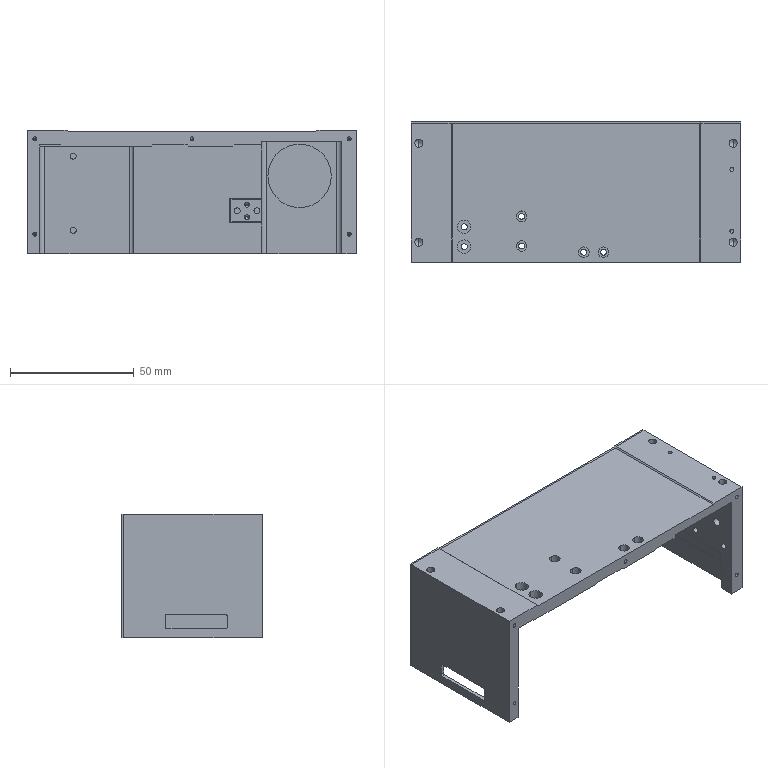NC program | NX | posted with a generic post | part box 133 x 56.74 x 50 mm
Lines 1 to 301 of 22463:
N10 G17 G21 G94 G90
(FLOOR_WALL_COPY_1 , TOOL : D10)
N12 T10 M6
N14 G54
N16 G17 G0 G90 X-74.5 Y28.367 B0. C0. S9500 M3
N18 G43 Z30. H10
N20 Z7.51
N22 G94 G1 Z4.51 F1250.
N24 X-71.5
N26 X71.5
N28 Y20.833
N30 X-71.5
N32 Y13.299
N34 X71.5
N36 Y5.765
N38 X-71.5
N40 Y-1.768
N42 X71.5
N44 Y-9.302
N46 X-71.5
N48 Y-16.836
N50 X71.5
N52 Y-24.37
N54 X-71.5
N56 X-74.5
N58 Z7.51
N60 G0 Z30.
N62 Y28.367
N64 Z7.02
N66 G1 Z4.02
N68 X-71.5
N70 X71.5
N72 Y20.833
N74 X-71.5
N76 Y13.299
N78 X71.5
N80 Y5.765
N82 X-71.5
N84 Y-1.768
N86 X71.5
N88 Y-9.302
N90 X-71.5
N92 Y-16.836
N94 X71.5
N96 Y-24.37
N98 X-71.5
N100 X-74.5
N102 Z7.02
N104 G0 Z30.
N106 Y28.367
N108 Z6.53
N110 G1 Z3.53
N112 X-71.5
N114 X71.5
N116 Y20.833
N118 X-71.5
N120 Y13.299
N122 X71.5
N124 Y5.765
N126 X-71.5
N128 Y-1.768
N130 X71.5
N132 Y-9.302
N134 X-71.5
N136 Y-16.836
N138 X71.5
N140 Y-24.37
N142 X-71.5
N144 X-74.5
N146 Z6.53
N148 G0 Z30.
N150 Y28.367
N152 Z6.04
N154 G1 Z3.04
N156 X-71.5
N158 X71.5
N160 Y20.833
N162 X-71.5
N164 Y13.299
N166 X71.5
N168 Y5.765
N170 X-71.5
N172 Y-1.768
N174 X71.5
N176 Y-9.302
N178 X-71.5
N180 Y-16.836
N182 X71.5
N184 Y-24.37
N186 X-71.5
N188 X-74.5
N190 Z6.04
N192 G0 Z30.
N194 Y28.367
N196 Z5.55
N198 G1 Z2.55
N200 X-71.5
N202 X71.5
N204 Y20.833
N206 X-71.5
N208 Y13.299
N210 X71.5
N212 Y5.765
N214 X-71.5
N216 Y-1.768
N218 X71.5
N220 Y-9.302
N222 X-71.5
N224 Y-16.836
N226 X71.5
N228 Y-24.37
N230 X-71.5
N232 X-74.5
N234 Z5.55
N236 G0 Z30.
N238 Y28.367
N240 Z5.06
N242 G1 Z2.06
N244 X-71.5
N246 X71.5
N248 Y20.833
N250 X-71.5
N252 Y13.299
N254 X71.5
N256 Y5.765
N258 X-71.5
N260 Y-1.768
N262 X71.5
N264 Y-9.302
N266 X-71.5
N268 Y-16.836
N270 X71.5
N272 Y-24.37
N274 X-71.5
N276 X-74.5
N278 Z5.06
N280 G0 Z30.
N282 Y28.367
N284 Z4.57
N286 G1 Z1.57
N288 X-71.5
N290 X71.5
N292 Y20.833
N294 X-71.5
N296 Y13.299
N298 X71.5
N300 Y5.765
N302 X-71.5
N304 Y-1.768
N306 X71.5
N308 Y-9.302
N310 X-71.5
N312 Y-16.836
N314 X71.5
N316 Y-24.37
N318 X-71.5
N320 X-74.5
N322 Z4.57
N324 G0 Z30.
N326 Y28.367
N328 Z4.08
N330 G1 Z1.08
N332 X-71.5
N334 X71.5
N336 Y20.833
N338 X-71.5
N340 Y13.299
N342 X71.5
N344 Y5.765
N346 X-71.5
N348 Y-1.768
N350 X71.5
N352 Y-9.302
N354 X-71.5
N356 Y-16.836
N358 X71.5
N360 Y-24.37
N362 X-71.5
N364 X-74.5
N366 Z4.08
N368 G0 Z30.
N370 Y28.367
N372 Z3.59
N374 G1 Z0.59
N376 X-71.5
N378 X71.5
N380 Y20.833
N382 X-71.5
N384 Y13.299
N386 X71.5
N388 Y5.765
N390 X-71.5
N392 Y-1.768
N394 X71.5
N396 Y-9.302
N398 X-71.5
N400 Y-16.836
N402 X71.5
N404 Y-24.37
N406 X-71.5
N408 X-74.5
N410 Z3.59
N412 G0 Z30.
N414 Y28.367
N416 Z3.1
N418 G1 Z0.1
N420 X-71.5
N422 X71.5
N424 Y20.833
N426 X-71.5
N428 Y13.299
N430 X71.5
N432 Y5.765
N434 X-71.5
N436 Y-1.768
N438 X71.5
N440 Y-9.302
N442 X-71.5
N444 Y-16.836
N446 X71.5
N448 Y-24.37
N450 X-71.5
N452 X-74.5
N454 Z3.1
N456 G0 Z30.
N458 M5
(FLOOR_WALL_COPY_2 , TOOL : D10JING)
N460 T09 M6
N462 G54
N464 G17 G0 G90 X-74.5 Y28.367 B0. C0. S9500 M3
N466 G43 Z30. H9
N468 Z3.
N470 G94 G1 Z0. F1250.
N472 X-71.5
N474 X71.5
N476 Y23.573
N478 X-71.5
N480 Y18.778
N482 X71.5
N484 Y13.984
N486 X-71.5
N488 Y9.19
N490 X71.5
N492 Y4.396
N494 X-71.5
N496 Y-0.399
N498 X71.5
N500 Y-5.193
N502 X-71.5
N504 Y-9.987
N506 X71.5
N508 Y-14.781
N510 X-71.5
N512 Y-19.576
N514 X71.5
N516 Y-24.37
N518 X-71.5
N520 X-74.5
N522 Z3.
N524 G0 Z30.
N526 M5
(DRILLING_COPY_1_COPY , TOOL : D6A45)
N528 T07 M6
N530 G54
N532 G17 G0 G90 X63.5 Y-25.37 B0. C0. S5000 M3
N534 G43 Z30. H7
N536 G94 G81 G98 Z-1. F250. R3.
N538 Y24.63
N540 X0.
N542 X-63.5
N544 X-63. Y-0.87
N546 Y-7.87
N548 X-63.5 Y-25.37
N550 G80
N552 G0 X-63.5 Y-25.37 Z30.
N554 M5
(DRILLING_COPY_COPY_COPY_1 , TOOL : 1.6ZT)
N556 T14 M6
N558 G54
N560 G17 G0 G90 X63.5 Y-25.37 B0. C0. S2000 M3
N562 G43 Z30. H14
N564 G94 G83 G98 Z-5.2 F150. Q2. R3.
N566 Y24.63
N568 X0.
N570 X-63.5
N572 X-63. Y-0.87 Z-22.52
N574 Y-7.87
N576 X-63.5 Y-25.37 Z-5.2
N578 G80
N580 G0 X-63.5 Y-25.37 Z30.
N582 M5